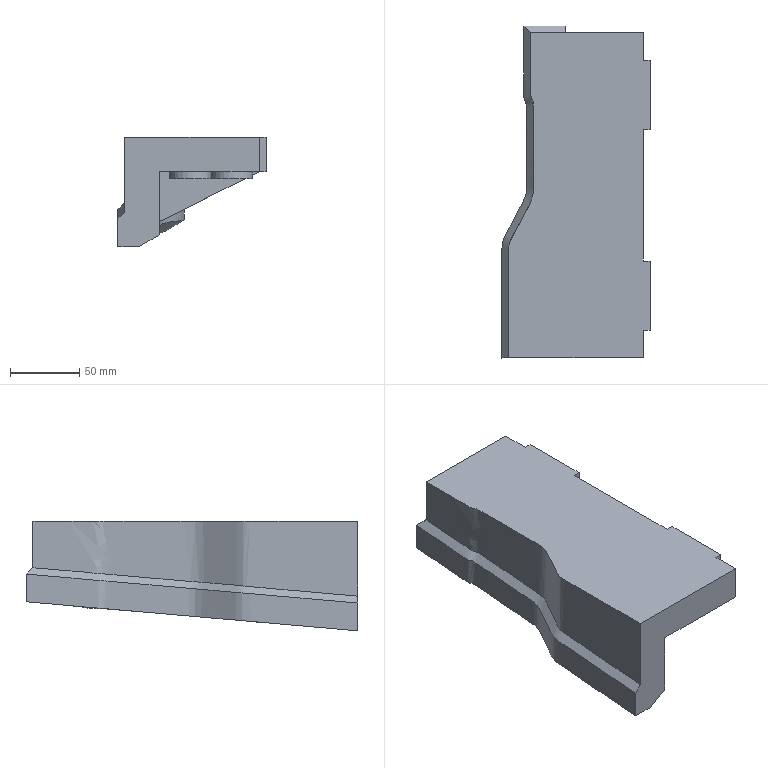Part | NX | features solid 2 | 1 solid | 36 faces | box 107.276 x 240 x 79.261 mm | volume 848822 mm3 | plane 25 | spline 6 | cylinder 5 | commonest cylinder face diameters 30 x5